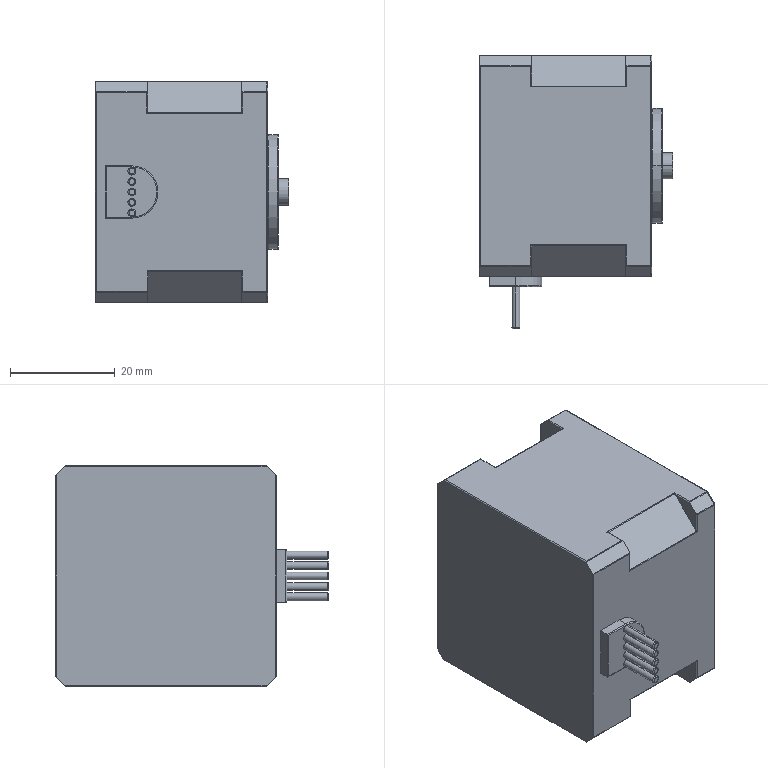Part | SolidWorks | features Revolution 6, ICE 5, HoleWzd 2, Extrusion 1, Fillet 1 | 1 solid | 156 faces | box 37 x 52.3 x 42.3 mm | volume 58361 mm3 | cylinder 79 | plane 42 | torus 27 | sphere 8 | commonest cylinder face diameters 0.4 x54 1.5 x10 3 x8 5 x2 12 x2 22 x2